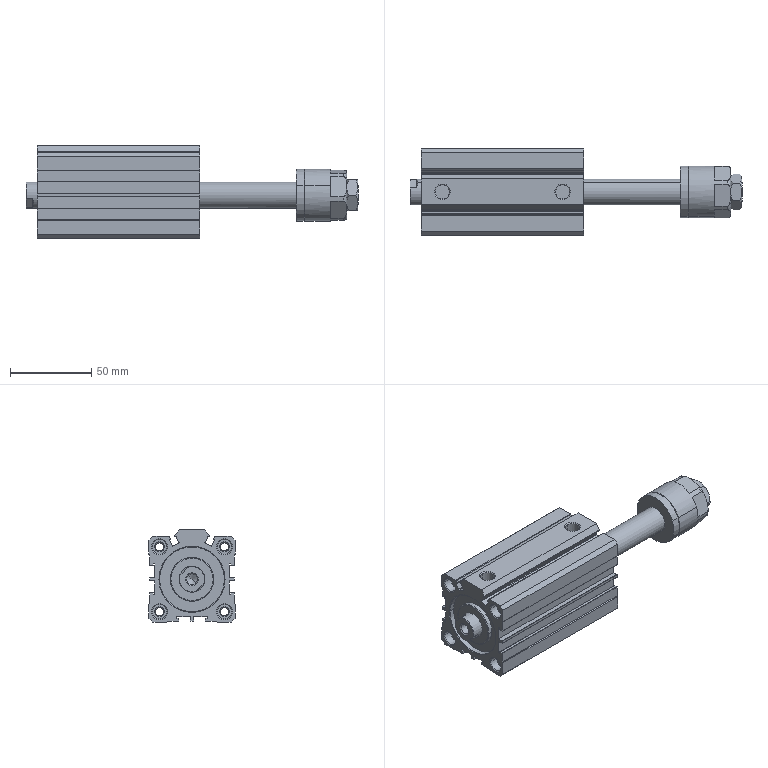Part | SolidWorks | features CompositeCurve 1 | 4 solids | 317 faces | box 204.5 x 53 x 57 mm | volume 221430 mm3 | plane 123 | cylinder 112 | cone 76 | spline 6 | commonest cylinder face diameters 0.4 x35 9 x16 0.8 x15 4.917 x8 16 x8 40 x8